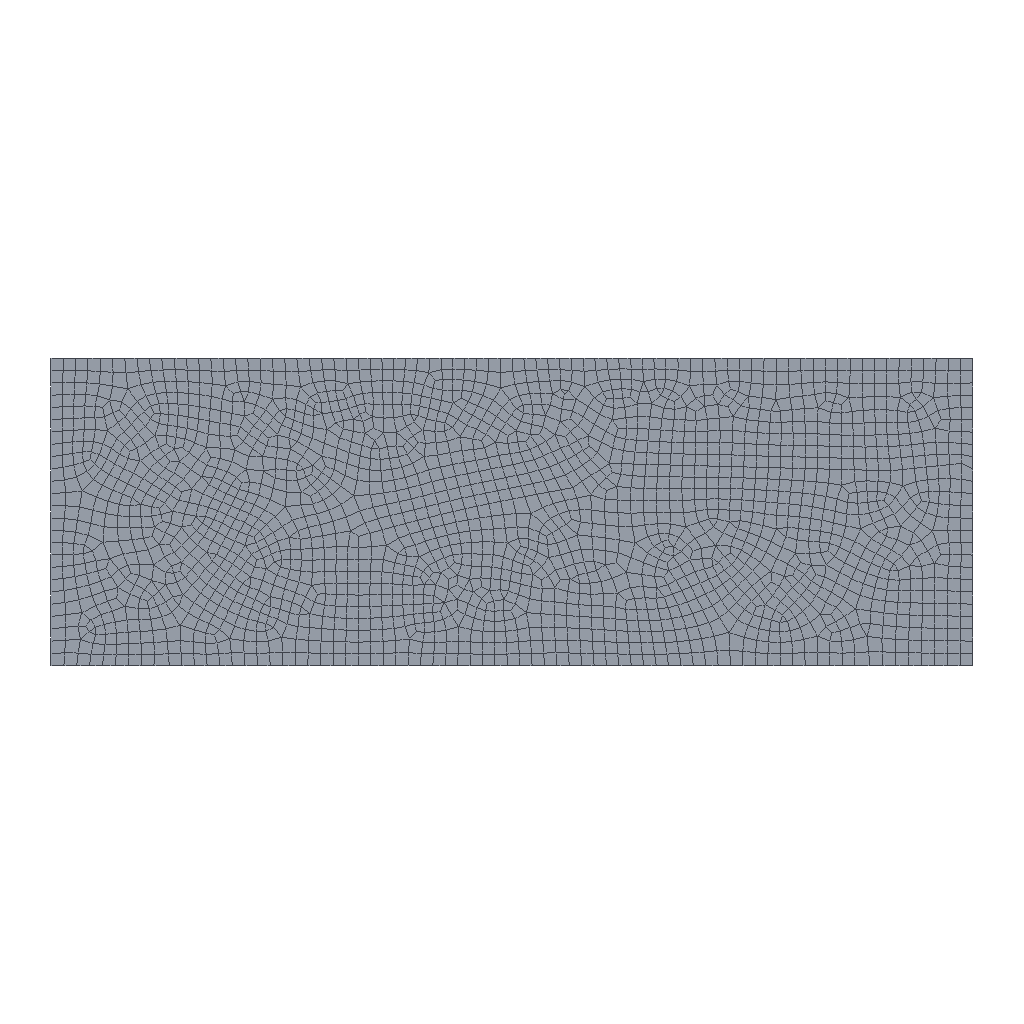Simulation study | abaqus
Set-up summary:
category,name,step,type,value,unit,region
solver,abaqus
solver,version,,,Abaqus/Explicit 2020
units,not stated in the deck,,not stated
analysis,deck,,transient,transient
load_step,Step-1,Step-1,transient
load_step,requested,,,1
mesh,nodes,,,2342
mesh,elements,,,2270
element_type,CPS3,,plane,57
element_type,CPS4R,,plane,2151
element_type,COH2D4,,cohesive,62
load,load commands in deck,,count,1
bc,support commands in deck,,count,1
material,COH,,in results
material,MATERIAL-1,,in results
check,setup vs results,,match,"per instance, exact: element labels, types and connectivity; labels of the nodes the elements use; coordinates of those nodes at SINGLE_PRECISION in 1 of 1 instance(s)"
Abaqus input file, long lists of numbers shortened:
*Heading
** Job name: Job-1 Model name: Model-1
** Generated by: Abaqus/CAE 2020
*Preprint, echo=NO, model=NO, history=NO, contact=NO
**
** PARTS
**
*Part, name=Part-1
*Node
      1,         584.,           0.
      2,         568.,           0.
** (2340 more lines like these left out)
*Element, type=CPS3
 1, 1809, 1853, 1879
 2, 2048, 1722, 1882
** (55 more lines like these left out)
*Element, type=CPS4R
  58,  479,    1,  789, 2012
  59, 2012,  619,   12,  479
** (2149 more lines like these left out)
*Element, type=COH2D4
2209, 2281,   86,   86,  580
2210, 2282, 2281,  580,  579
** (60 more lines like these left out)
*Nset, nset=Set-5, generate
    1,  2342,     1
*Elset, elset=Set-5, generate
    1,  2208,     1
*Elset, elset=CohesiveSeam-1-Elements, generate
 2209,  2270,     1
*Nset, nset=CohesiveSeam-1-TopNodes
   60,   61,   62,   63,   64,   72,   73,   74,   84,   85,   86,  545,  546,  547,  548,  549
  550,  551,  562,  563,  577,  578,  579,  580, 2286, 2287, 2288, 2289, 2290, 2291, 2292, 2293
** (3 more lines like these left out)
*Nset, nset=CohesiveSeam-1-BottomNodes
   64,   65,   66,   67,   68,   69,   70,   71,   72,   74,   75,   76,   77,   78,   79,   80
   81,   82,   83,   84,   86,  552,  553,  554,  555,  556,  557,  558,  559,  560,  561,  564
** (3 more lines like these left out)
*Nset, nset=CohesiveSeam-1-MidNodes
 86,
*Elset, elset=__PickedSurf5_S1, internal
  148,  151,  385,  386,  388,  413,  444,  454,  488,  506,  719,  914, 1025, 2209, 2210, 2211
 2212, 2213, 2214, 2238, 2239, 2240, 2241, 2260, 2261, 2262, 2263, 2264, 2265, 2266, 2267, 2268
** (1 more lines like these left out)
*Elset, elset=__PickedSurf5_S3, internal
  147,  149,  150,  389,  390,  392,  393,  394,  395,  429,  450,  753,  913,  916,  918,  919
  971,  986, 1014, 1017, 1022, 2215, 2216, 2217, 2218, 2219, 2220, 2221, 2222, 2223, 2224, 2225
** (2 more lines like these left out)
*Elset, elset=__PickedSurf5_S4, internal
 108, 109, 111, 144, 190, 191, 196, 387, 399, 400, 404, 405, 406, 410, 412, 487
 528, 544, 552, 579, 692, 922, 927, 928, 930, 931
*Elset, elset=__PickedSurf5_S2, internal
   97,   98,   99,  143,  398,  409,  463,  464,  466,  491,  561,  570,  590,  924,  925,  926
  929,  932,  933, 1035, 1042, 1045
*Surface, type=ELEMENT, name=_PickedSurf5, internal
__PickedSurf5_S1, S1
__PickedSurf5_S3, S3
__PickedSurf5_S4, S4
__PickedSurf5_S2, S2
*Elset, elset=_CohesiveSeam-1-TopSurf_S3, internal, generate
 2209,  2270,     1
*Surface, type=ELEMENT, name=CohesiveSeam-1-TopSurf
_CohesiveSeam-1-TopSurf_S3, S3
*Elset, elset=_CohesiveSeam-1-BottomSurf_S1, internal, generate
 2209,  2270,     1
*Surface, type=ELEMENT, name=CohesiveSeam-1-BottomSurf
_CohesiveSeam-1-BottomSurf_S1, S1
** Section: Section-1
*Solid Section, elset=Set-5, material=Material-1
,
** Section: cohaa
*Cohesive Section, elset=CohesiveSeam-1-Elements, controls=EC-1, material=coh, response=TRACTION SEPARATION
,
*End Part
**
**
** ASSEMBLY
**
*Assembly, name=Assembly
**
*Instance, name=Part-1-1, part=Part-1
*End Instance
**
*Nset, nset=Set-1, instance=Part-1-1
  53,  54, 104, 105
*Elset, elset=Set-1, instance=Part-1-1
 271, 580
*Elset, elset=_Surf-1_S1, internal, instance=Part-1-1
 186, 192, 197, 203, 204, 209, 210, 214, 219, 226, 233, 240, 241, 246, 247, 250
 988, 990, 993, 995, 997
*Elset, elset=_Surf-1_S3, internal, instance=Part-1-1
  861,  866,  869, 1001, 1003
*Surface, type=ELEMENT, name=Surf-1
_Surf-1_S1, S1
_Surf-1_S3, S3
*End Assembly
**
** ELEMENT CONTROLS
**
*Section Controls, name=EC-1, ELEMENT DELETION=YES
1., 1., 1.
**
** MATERIALS
**
*Material, name=Material-1
*Density
 5.8e-09,
*Elastic
1000., 0.3
*Material, name=coh
*Damage Initiation, criterion=MAXS
8.,8.,8.
*Damage Evolution, type=DISPLACEMENT
 1e-11,
*Density
 5.8e-09,
*Elastic, type=TRACTION
1000.,1000.,1000.
**
** INTERACTION PROPERTIES
**
*Surface Interaction, name=IntProp-1
*Friction
 0.01,
*Surface Behavior, pressure-overclosure=HARD
** ----------------------------------------------------------------
**
** STEP: Step-1
**
*Step, name=Step-1, nlgeom=YES
*Dynamic, Explicit
, 0.1
*Bulk Viscosity
0.06, 1.2
**
** BOUNDARY CONDITIONS
**
** Name: BC-1 Type: 对称/反对称/完全固定
*Boundary
Set-1, ENCASTRE
**
** LOADS
**
** Name: Load-1   Type: Pressure
*Dsload
Surf-1, P, 5.
**
** INTERACTIONS
**
** Interaction: Int-1
*Contact, op=NEW
*Contact Inclusions, ALL EXTERIOR
*Contact Property Assignment
 ,  , IntProp-1
**
** OUTPUT REQUESTS
**
*Restart, write, number interval=1, time marks=NO
**
** FIELD OUTPUT: F-Output-1
**
*Output, field, number interval=50
*Node Output
A, RF, U, V
*Element Output, directions=YES
E, EVF, LE, MISES, MISESMAX, MISESONLY, PE, PEEQ, PEEQVAVG, PEVAVG, S, SDEG, SEQUT, STATUS, SVAVG, YIELDPOT
*Contact Output
CDISP, CSTRESS
**
** HISTORY OUTPUT: H-Output-1
**
*Output, history, variable=PRESELECT
*End Step
Results summary:
result,step,Step-1,completed,increments=21920 time=0.1/0.1
result,analysis,,,transient
result,last_loadstep,,,1
result,primary field,,,U
result,reaction total,,FX,57.795,model units
result,reaction total,,FY,1422.133,model units
result,reaction total,,FZ,0.0,model units